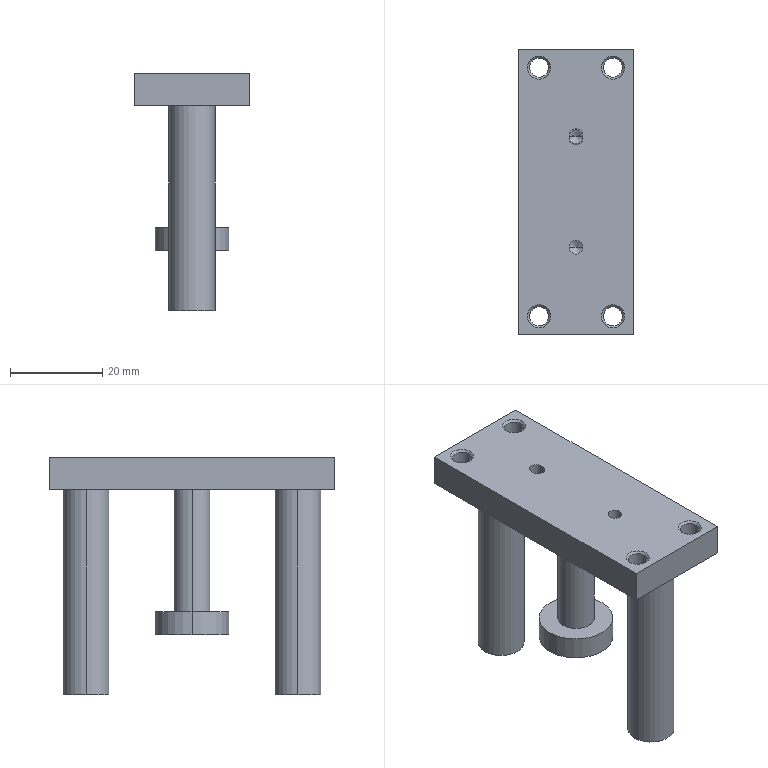Part | SolidWorks | features ICE 4, RevCut 4, RefAxis 3, HoleWzd 2, 3DProfileFeature 1, Extrusion 1, Revolution 1 | 1 solid | 56 faces | box 25 x 62 x 51.5 mm | volume 19698 mm3 | cylinder 22 | cone 20 | plane 14 | commonest cylinder face diameters 4.134 x8 3 x6 10 x4 8 x2 16 x2
STEP:
#1=CARTESIAN_POINT('',(-5.933,27.,12.567));
#2=VERTEX_POINT('',#1);
#3=CARTESIAN_POINT('',(-10.067,27.,12.567));
#4=VERTEX_POINT('',#3);
#5=CARTESIAN_POINT('',(-8.,27.,12.567));
#6=DIRECTION('',(0.,0.,-1.));
#7=DIRECTION('',(-1.,0.,0.));
#8=AXIS2_PLACEMENT_3D('',#5,#6,#7);
#9=CIRCLE('',#8,2.067);
#10=EDGE_CURVE('',#2,#4,#9,.T.);
#11=ORIENTED_EDGE('',*,*,#10,.T.);
#12=CARTESIAN_POINT('',(-10.5,27.,13.));
#13=VERTEX_POINT('',#12);
#14=CARTESIAN_POINT('',(-10.5,27.,13.));
#15=DIRECTION('',(-0.7071,0.,0.7071));
#16=VECTOR('',#15,1000.);
#17=LINE('',#14,#16);
#18=EDGE_CURVE('',#4,#13,#17,.T.);
#19=ORIENTED_EDGE('',*,*,#18,.T.);
#20=CARTESIAN_POINT('',(-5.5,27.,13.));
#21=VERTEX_POINT('',#20);
#22=CARTESIAN_POINT('',(-8.,27.,13.));
#23=DIRECTION('',(0.,0.,-1.));
#24=DIRECTION('',(-1.,0.,0.));
#25=AXIS2_PLACEMENT_3D('',#22,#23,#24);
#26=CIRCLE('',#25,2.5);
#27=EDGE_CURVE('',#21,#13,#26,.T.);
#28=ORIENTED_EDGE('',*,*,#27,.F.);
#29=CARTESIAN_POINT('',(-5.5,27.,13.));
#30=DIRECTION('',(0.7071,0.,0.7071));
#31=VECTOR('',#30,1000.);
#32=LINE('',#29,#31);
#33=EDGE_CURVE('',#2,#21,#32,.T.);
#34=ORIENTED_EDGE('',*,*,#33,.F.);
#35=EDGE_LOOP('',(#11,#19,#28,#34));
#36=FACE_OUTER_BOUND('',#35,.T.);
#37=CARTESIAN_POINT('',(-8.,27.,13.));
#38=DIRECTION('',(0.,0.,1.));
#39=DIRECTION('',(1.,0.,0.));
#40=AXIS2_PLACEMENT_3D('',#37,#38,#39);
#41=CONICAL_SURFACE('',#40,2.5,0.7854);
#42=ADVANCED_FACE('',(#36),#41,.F.);
#43=ORIENTED_EDGE('',*,*,#10,.F.);
#44=CARTESIAN_POINT('',(-5.933,27.,6.433));
#45=VERTEX_POINT('',#44);
#46=CARTESIAN_POINT('',(-5.933,27.,13.));
#47=DIRECTION('',(0.,0.,-1.));
#48=VECTOR('',#47,1000.);
#49=LINE('',#46,#48);
#50=EDGE_CURVE('',#2,#45,#49,.T.);
#51=ORIENTED_EDGE('',*,*,#50,.T.);
#52=CARTESIAN_POINT('',(-10.067,27.,6.433));
#53=VERTEX_POINT('',#52);
#54=CARTESIAN_POINT('',(-8.,27.,6.433));
#55=DIRECTION('',(0.,0.,-1.));
#56=DIRECTION('',(-1.,0.,0.));
#57=AXIS2_PLACEMENT_3D('',#54,#55,#56);
#58=CIRCLE('',#57,2.067);
#59=EDGE_CURVE('',#45,#53,#58,.T.);
#60=ORIENTED_EDGE('',*,*,#59,.T.);
#61=CARTESIAN_POINT('',(-10.067,27.,13.));
#62=DIRECTION('',(0.,0.,-1.));
#63=VECTOR('',#62,1000.);
#64=LINE('',#61,#63);
#65=EDGE_CURVE('',#4,#53,#64,.T.);
#66=ORIENTED_EDGE('',*,*,#65,.F.);
#67=EDGE_LOOP('',(#43,#51,#60,#66));
#68=FACE_OUTER_BOUND('',#67,.T.);
#69=CARTESIAN_POINT('',(-8.,27.,13.));
#70=DIRECTION('',(0.,0.,-1.));
#71=DIRECTION('',(-1.,0.,0.));
#72=AXIS2_PLACEMENT_3D('',#69,#70,#71);
#73=CYLINDRICAL_SURFACE('',#72,2.067);
#74=ADVANCED_FACE('',(#68),#73,.F.);
#75=ORIENTED_EDGE('',*,*,#59,.F.);
#76=CARTESIAN_POINT('',(-5.5,27.,6.));
#77=VERTEX_POINT('',#76);
#78=CARTESIAN_POINT('',(-5.933,27.,6.433));
#79=DIRECTION('',(0.7071,0.,-0.7071));
#80=VECTOR('',#79,1000.);
#81=LINE('',#78,#80);
#82=EDGE_CURVE('',#45,#77,#81,.T.);
#83=ORIENTED_EDGE('',*,*,#82,.T.);
#84=CARTESIAN_POINT('',(-10.5,27.,6.));
#85=VERTEX_POINT('',#84);
#86=CARTESIAN_POINT('',(-8.,27.,6.));
#87=DIRECTION('',(0.,0.,-1.));
#88=DIRECTION('',(-1.,0.,0.));
#89=AXIS2_PLACEMENT_3D('',#86,#87,#88);
#90=CIRCLE('',#89,2.5);
#91=EDGE_CURVE('',#77,#85,#90,.T.);
#92=ORIENTED_EDGE('',*,*,#91,.T.);
#93=CARTESIAN_POINT('',(-10.067,27.,6.433));
#94=DIRECTION('',(-0.7071,0.,-0.7071));
#95=VECTOR('',#94,1000.);
#96=LINE('',#93,#95);
#97=EDGE_CURVE('',#53,#85,#96,.T.);
#98=ORIENTED_EDGE('',*,*,#97,.F.);
#99=EDGE_LOOP('',(#75,#83,#92,#98));
#100=FACE_OUTER_BOUND('',#99,.T.);
#101=CARTESIAN_POINT('',(-8.,27.,6.433));
#102=DIRECTION('',(0.,0.,-1.));
#103=DIRECTION('',(-1.,0.,0.));
#104=AXIS2_PLACEMENT_3D('',#101,#102,#103);
#105=CONICAL_SURFACE('',#104,2.067,0.7854);
#106=ADVANCED_FACE('',(#100),#105,.F.);
#107=CARTESIAN_POINT('',(10.067,27.,12.567));
#108=VERTEX_POINT('',#107);
#109=CARTESIAN_POINT('',(5.933,27.,12.567));
#110=VERTEX_POINT('',#109);
#111=CARTESIAN_POINT('',(8.,27.,12.567));
#112=DIRECTION('',(0.,0.,-1.));
#113=DIRECTION('',(-1.,0.,0.));
#114=AXIS2_PLACEMENT_3D('',#111,#112,#113);
#115=CIRCLE('',#114,2.067);
#116=EDGE_CURVE('',#108,#110,#115,.T.);
#117=ORIENTED_EDGE('',*,*,#116,.T.);
#118=CARTESIAN_POINT('',(5.5,27.,13.));
#119=VERTEX_POINT('',#118);
#120=CARTESIAN_POINT('',(5.5,27.,13.));
#121=DIRECTION('',(-0.7071,0.,0.7071));
#122=VECTOR('',#121,1000.);
#123=LINE('',#120,#122);
#124=EDGE_CURVE('',#110,#119,#123,.T.);
#125=ORIENTED_EDGE('',*,*,#124,.T.);
#126=CARTESIAN_POINT('',(10.5,27.,13.));
#127=VERTEX_POINT('',#126);
#128=CARTESIAN_POINT('',(8.,27.,13.));
#129=DIRECTION('',(0.,0.,-1.));
#130=DIRECTION('',(-1.,0.,0.));
#131=AXIS2_PLACEMENT_3D('',#128,#129,#130);
#132=CIRCLE('',#131,2.5);
#133=EDGE_CURVE('',#127,#119,#132,.T.);
#134=ORIENTED_EDGE('',*,*,#133,.F.);
#135=CARTESIAN_POINT('',(10.5,27.,13.));
#136=DIRECTION('',(0.7071,0.,0.7071));
#137=VECTOR('',#136,1000.);
#138=LINE('',#135,#137);
#139=EDGE_CURVE('',#108,#127,#138,.T.);
#140=ORIENTED_EDGE('',*,*,#139,.F.);
#141=EDGE_LOOP('',(#117,#125,#134,#140));
#142=FACE_OUTER_BOUND('',#141,.T.);
#143=CARTESIAN_POINT('',(8.,27.,13.));
#144=DIRECTION('',(0.,0.,1.));
#145=DIRECTION('',(1.,0.,0.));
#146=AXIS2_PLACEMENT_3D('',#143,#144,#145);
#147=CONICAL_SURFACE('',#146,2.5,0.7854);
#148=ADVANCED_FACE('',(#142),#147,.F.);
#149=ORIENTED_EDGE('',*,*,#116,.F.);
#150=CARTESIAN_POINT('',(10.067,27.,6.433));
#151=VERTEX_POINT('',#150);
#152=CARTESIAN_POINT('',(10.067,27.,13.));
#153=DIRECTION('',(0.,0.,-1.));
#154=VECTOR('',#153,1000.);
#155=LINE('',#152,#154);
#156=EDGE_CURVE('',#108,#151,#155,.T.);
#157=ORIENTED_EDGE('',*,*,#156,.T.);
#158=CARTESIAN_POINT('',(5.933,27.,6.433));
#159=VERTEX_POINT('',#158);
#160=CARTESIAN_POINT('',(8.,27.,6.433));
#161=DIRECTION('',(0.,0.,-1.));
#162=DIRECTION('',(-1.,0.,0.));
#163=AXIS2_PLACEMENT_3D('',#160,#161,#162);
#164=CIRCLE('',#163,2.067);
#165=EDGE_CURVE('',#151,#159,#164,.T.);
#166=ORIENTED_EDGE('',*,*,#165,.T.);
#167=CARTESIAN_POINT('',(5.933,27.,13.));
#168=DIRECTION('',(0.,0.,-1.));
#169=VECTOR('',#168,1000.);
#170=LINE('',#167,#169);
#171=EDGE_CURVE('',#110,#159,#170,.T.);
#172=ORIENTED_EDGE('',*,*,#171,.F.);
#173=EDGE_LOOP('',(#149,#157,#166,#172));
#174=FACE_OUTER_BOUND('',#173,.T.);
#175=CARTESIAN_POINT('',(8.,27.,13.));
#176=DIRECTION('',(0.,0.,-1.));
#177=DIRECTION('',(-1.,0.,0.));
#178=AXIS2_PLACEMENT_3D('',#175,#176,#177);
#179=CYLINDRICAL_SURFACE('',#178,2.067);
#180=ADVANCED_FACE('',(#174),#179,.F.);
#181=ORIENTED_EDGE('',*,*,#165,.F.);
#182=CARTESIAN_POINT('',(10.5,27.,6.));
#183=VERTEX_POINT('',#182);
#184=CARTESIAN_POINT('',(10.067,27.,6.433));
#185=DIRECTION('',(0.7071,0.,-0.7071));
#186=VECTOR('',#185,1000.);
#187=LINE('',#184,#186);
#188=EDGE_CURVE('',#151,#183,#187,.T.);
#189=ORIENTED_EDGE('',*,*,#188,.T.);
#190=CARTESIAN_POINT('',(5.5,27.,6.));
#191=VERTEX_POINT('',#190);
#192=CARTESIAN_POINT('',(8.,27.,6.));
#193=DIRECTION('',(0.,0.,-1.));
#194=DIRECTION('',(-1.,0.,0.));
#195=AXIS2_PLACEMENT_3D('',#192,#193,#194);
#196=CIRCLE('',#195,2.5);
#197=EDGE_CURVE('',#183,#191,#196,.T.);
#198=ORIENTED_EDGE('',*,*,#197,.T.);
#199=CARTESIAN_POINT('',(5.933,27.,6.433));
#200=DIRECTION('',(-0.7071,0.,-0.7071));
#201=VECTOR('',#200,1000.);
#202=LINE('',#199,#201);
#203=EDGE_CURVE('',#159,#191,#202,.T.);
#204=ORIENTED_EDGE('',*,*,#203,.F.);
#205=EDGE_LOOP('',(#181,#189,#198,#204));
#206=FACE_OUTER_BOUND('',#205,.T.);
#207=CARTESIAN_POINT('',(8.,27.,6.433));
#208=DIRECTION('',(0.,0.,-1.));
#209=DIRECTION('',(-1.,0.,0.));
#210=AXIS2_PLACEMENT_3D('',#207,#208,#209);
#211=CONICAL_SURFACE('',#210,2.067,0.7854);
#212=ADVANCED_FACE('',(#206),#211,.F.);
#213=CARTESIAN_POINT('',(-5.933,-27.,12.567));
#214=VERTEX_POINT('',#213);
#215=CARTESIAN_POINT('',(-10.067,-27.,12.567));
#216=VERTEX_POINT('',#215);
#217=CARTESIAN_POINT('',(-8.,-27.,12.567));
#218=DIRECTION('',(0.,0.,-1.));
#219=DIRECTION('',(-1.,0.,0.));
#220=AXIS2_PLACEMENT_3D('',#217,#218,#219);
#221=CIRCLE('',#220,2.067);
#222=EDGE_CURVE('',#214,#216,#221,.T.);
#223=ORIENTED_EDGE('',*,*,#222,.T.);
#224=CARTESIAN_POINT('',(-10.5,-27.,13.));
#225=VERTEX_POINT('',#224);
#226=CARTESIAN_POINT('',(-10.5,-27.,13.));
#227=DIRECTION('',(-0.7071,0.,0.7071));
#228=VECTOR('',#227,1000.);
#229=LINE('',#226,#228);
#230=EDGE_CURVE('',#216,#225,#229,.T.);
#231=ORIENTED_EDGE('',*,*,#230,.T.);
#232=CARTESIAN_POINT('',(-5.5,-27.,13.));
#233=VERTEX_POINT('',#232);
#234=CARTESIAN_POINT('',(-8.,-27.,13.));
#235=DIRECTION('',(0.,0.,-1.));
#236=DIRECTION('',(-1.,0.,0.));
#237=AXIS2_PLACEMENT_3D('',#234,#235,#236);
#238=CIRCLE('',#237,2.5);
#239=EDGE_CURVE('',#233,#225,#238,.T.);
#240=ORIENTED_EDGE('',*,*,#239,.F.);
#241=CARTESIAN_POINT('',(-5.5,-27.,13.));
#242=DIRECTION('',(0.7071,0.,0.7071));
#243=VECTOR('',#242,1000.);
#244=LINE('',#241,#243);
#245=EDGE_CURVE('',#214,#233,#244,.T.);
#246=ORIENTED_EDGE('',*,*,#245,.F.);
#247=EDGE_LOOP('',(#223,#231,#240,#246));
#248=FACE_OUTER_BOUND('',#247,.T.);
#249=CARTESIAN_POINT('',(-8.,-27.,13.));
#250=DIRECTION('',(0.,0.,1.));
#251=DIRECTION('',(1.,0.,0.));
#252=AXIS2_PLACEMENT_3D('',#249,#250,#251);
#253=CONICAL_SURFACE('',#252,2.5,0.7854);
#254=ADVANCED_FACE('',(#248),#253,.F.);
#255=ORIENTED_EDGE('',*,*,#222,.F.);
#256=CARTESIAN_POINT('',(-5.933,-27.,6.433));
#257=VERTEX_POINT('',#256);
#258=CARTESIAN_POINT('',(-5.933,-27.,13.));
#259=DIRECTION('',(0.,0.,-1.));
#260=VECTOR('',#259,1000.);
#261=LINE('',#258,#260);
#262=EDGE_CURVE('',#214,#257,#261,.T.);
#263=ORIENTED_EDGE('',*,*,#262,.T.);
#264=CARTESIAN_POINT('',(-10.067,-27.,6.433));
#265=VERTEX_POINT('',#264);
#266=CARTESIAN_POINT('',(-8.,-27.,6.433));
#267=DIRECTION('',(0.,0.,-1.));
#268=DIRECTION('',(-1.,0.,0.));
#269=AXIS2_PLACEMENT_3D('',#266,#267,#268);
#270=CIRCLE('',#269,2.067);
#271=EDGE_CURVE('',#257,#265,#270,.T.);
#272=ORIENTED_EDGE('',*,*,#271,.T.);
#273=CARTESIAN_POINT('',(-10.067,-27.,13.));
#274=DIRECTION('',(0.,0.,-1.));
#275=VECTOR('',#274,1000.);
#276=LINE('',#273,#275);
#277=EDGE_CURVE('',#216,#265,#276,.T.);
#278=ORIENTED_EDGE('',*,*,#277,.F.);
#279=EDGE_LOOP('',(#255,#263,#272,#278));
#280=FACE_OUTER_BOUND('',#279,.T.);
#281=CARTESIAN_POINT('',(-8.,-27.,13.));
#282=DIRECTION('',(0.,0.,-1.));
#283=DIRECTION('',(-1.,0.,0.));
#284=AXIS2_PLACEMENT_3D('',#281,#282,#283);
#285=CYLINDRICAL_SURFACE('',#284,2.067);
#286=ADVANCED_FACE('',(#280),#285,.F.);
#287=ORIENTED_EDGE('',*,*,#271,.F.);
#288=CARTESIAN_POINT('',(-5.5,-27.,6.));
#289=VERTEX_POINT('',#288);
#290=CARTESIAN_POINT('',(-5.933,-27.,6.433));
#291=DIRECTION('',(0.7071,0.,-0.7071));
#292=VECTOR('',#291,1000.);
#293=LINE('',#290,#292);
#294=EDGE_CURVE('',#257,#289,#293,.T.);
#295=ORIENTED_EDGE('',*,*,#294,.T.);
#296=CARTESIAN_POINT('',(-10.5,-27.,6.));
#297=VERTEX_POINT('',#296);
#298=CARTESIAN_POINT('',(-8.,-27.,6.));
#299=DIRECTION('',(0.,0.,-1.));
#300=DIRECTION('',(-1.,0.,0.));
#301=AXIS2_PLACEMENT_3D('',#298,#299,#300);
#302=CIRCLE('',#301,2.5);
#303=EDGE_CURVE('',#289,#297,#302,.T.);
#304=ORIENTED_EDGE('',*,*,#303,.T.);
#305=CARTESIAN_POINT('',(-10.067,-27.,6.433));
#306=DIRECTION('',(-0.7071,0.,-0.7071));
#307=VECTOR('',#306,1000.);
#308=LINE('',#305,#307);
#309=EDGE_CURVE('',#265,#297,#308,.T.);
#310=ORIENTED_EDGE('',*,*,#309,.F.);
#311=EDGE_LOOP('',(#287,#295,#304,#310));
#312=FACE_OUTER_BOUND('',#311,.T.);
#313=CARTESIAN_POINT('',(-8.,-27.,6.433));
#314=DIRECTION('',(0.,0.,-1.));
#315=DIRECTION('',(-1.,0.,0.));
#316=AXIS2_PLACEMENT_3D('',#313,#314,#315);
#317=CONICAL_SURFACE('',#316,2.067,0.7854);
#318=ADVANCED_FACE('',(#312),#317,.F.);
#319=CARTESIAN_POINT('',(10.067,-27.,12.567));
#320=VERTEX_POINT('',#319);
#321=CARTESIAN_POINT('',(5.933,-27.,12.567));
#322=VERTEX_POINT('',#321);
#323=CARTESIAN_POINT('',(8.,-27.,12.567));
#324=DIRECTION('',(0.,0.,-1.));
#325=DIRECTION('',(-1.,0.,0.));
#326=AXIS2_PLACEMENT_3D('',#323,#324,#325);
#327=CIRCLE('',#326,2.067);
#328=EDGE_CURVE('',#320,#322,#327,.T.);
#329=ORIENTED_EDGE('',*,*,#328,.T.);
#330=CARTESIAN_POINT('',(5.5,-27.,13.));
#331=VERTEX_POINT('',#330);
#332=CARTESIAN_POINT('',(5.5,-27.,13.));
#333=DIRECTION('',(-0.7071,0.,0.7071));
#334=VECTOR('',#333,1000.);
#335=LINE('',#332,#334);
#336=EDGE_CURVE('',#322,#331,#335,.T.);
#337=ORIENTED_EDGE('',*,*,#336,.T.);
#338=CARTESIAN_POINT('',(10.5,-27.,13.));
#339=VERTEX_POINT('',#338);
#340=CARTESIAN_POINT('',(8.,-27.,13.));
#341=DIRECTION('',(0.,0.,-1.));
#342=DIRECTION('',(-1.,0.,0.));
#343=AXIS2_PLACEMENT_3D('',#340,#341,#342);
#344=CIRCLE('',#343,2.5);
#345=EDGE_CURVE('',#339,#331,#344,.T.);
#346=ORIENTED_EDGE('',*,*,#345,.F.);
#347=CARTESIAN_POINT('',(10.5,-27.,13.));
#348=DIRECTION('',(0.7071,0.,0.7071));
#349=VECTOR('',#348,1000.);
#350=LINE('',#347,#349);
#351=EDGE_CURVE('',#320,#339,#350,.T.);
#352=ORIENTED_EDGE('',*,*,#351,.F.);
#353=EDGE_LOOP('',(#329,#337,#346,#352));
#354=FACE_OUTER_BOUND('',#353,.T.);
#355=CARTESIAN_POINT('',(8.,-27.,13.));
#356=DIRECTION('',(0.,0.,1.));
#357=DIRECTION('',(1.,0.,0.));
#358=AXIS2_PLACEMENT_3D('',#355,#356,#357);
#359=CONICAL_SURFACE('',#358,2.5,0.7854);
#360=ADVANCED_FACE('',(#354),#359,.F.);
#361=ORIENTED_EDGE('',*,*,#328,.F.);
#362=CARTESIAN_POINT('',(10.067,-27.,6.433));
#363=VERTEX_POINT('',#362);
#364=CARTESIAN_POINT('',(10.067,-27.,13.));
#365=DIRECTION('',(0.,0.,-1.));
#366=VECTOR('',#365,1000.);
#367=LINE('',#364,#366);
#368=EDGE_CURVE('',#320,#363,#367,.T.);
#369=ORIENTED_EDGE('',*,*,#368,.T.);
#370=CARTESIAN_POINT('',(5.933,-27.,6.433));
#371=VERTEX_POINT('',#370);
#372=CARTESIAN_POINT('',(8.,-27.,6.433));
#373=DIRECTION('',(0.,0.,-1.));
#374=DIRECTION('',(-1.,0.,0.));
#375=AXIS2_PLACEMENT_3D('',#372,#373,#374);
#376=CIRCLE('',#375,2.067);
#377=EDGE_CURVE('',#363,#371,#376,.T.);
#378=ORIENTED_EDGE('',*,*,#377,.T.);
#379=CARTESIAN_POINT('',(5.933,-27.,13.));
#380=DIRECTION('',(0.,0.,-1.));
#381=VECTOR('',#380,1000.);
#382=LINE('',#379,#381);
#383=EDGE_CURVE('',#322,#371,#382,.T.);
#384=ORIENTED_EDGE('',*,*,#383,.F.);
#385=EDGE_LOOP('',(#361,#369,#378,#384));
#386=FACE_OUTER_BOUND('',#385,.T.);
#387=CARTESIAN_POINT('',(8.,-27.,13.));
#388=DIRECTION('',(0.,0.,-1.));
#389=DIRECTION('',(-1.,0.,0.));
#390=AXIS2_PLACEMENT_3D('',#387,#388,#389);
#391=CYLINDRICAL_SURFACE('',#390,2.067);
#392=ADVANCED_FACE('',(#386),#391,.F.);
#393=ORIENTED_EDGE('',*,*,#377,.F.);
#394=CARTESIAN_POINT('',(10.5,-27.,6.));
#395=VERTEX_POINT('',#394);
#396=CARTESIAN_POINT('',(10.067,-27.,6.433));
#397=DIRECTION('',(0.7071,0.,-0.7071));
#398=VECTOR('',#397,1000.);
#399=LINE('',#396,#398);
#400=EDGE_CURVE('',#363,#395,#399,.T.);
#401=ORIENTED_EDGE('',*,*,#400,.T.);
#402=CARTESIAN_POINT('',(5.5,-27.,6.));
#403=VERTEX_POINT('',#402);
#404=CARTESIAN_POINT('',(8.,-27.,6.));
#405=DIRECTION('',(0.,0.,-1.));
#406=DIRECTION('',(-1.,0.,0.));
#407=AXIS2_PLACEMENT_3D('',#404,#405,#406);
#408=CIRCLE('',#407,2.5);
#409=EDGE_CURVE('',#395,#403,#408,.T.);
#410=ORIENTED_EDGE('',*,*,#409,.T.);
#411=CARTESIAN_POINT('',(5.933,-27.,6.433));
#412=DIRECTION('',(-0.7071,0.,-0.7071));
#413=VECTOR('',#412,1000.);
#414=LINE('',#411,#413);
#415=EDGE_CURVE('',#371,#403,#414,.T.);
#416=ORIENTED_EDGE('',*,*,#415,.F.);
#417=EDGE_LOOP('',(#393,#401,#410,#416));
#418=FACE_OUTER_BOUND('',#417,.T.);
#419=CARTESIAN_POINT('',(8.,-27.,6.433));
#420=DIRECTION('',(0.,0.,-1.));
#421=DIRECTION('',(-1.,0.,0.));
#422=AXIS2_PLACEMENT_3D('',#419,#420,#421);
#423=CONICAL_SURFACE('',#422,2.067,0.7854);
#424=ADVANCED_FACE('',(#418),#423,.F.);
#425=CARTESIAN_POINT('',(-1.5,-12.,7.));
#426=VERTEX_POINT('',#425);
#427=CARTESIAN_POINT('',(1.5,-12.,7.));
#428=VERTEX_POINT('',#427);
#429=CARTESIAN_POINT('',(0.,-12.,7.));
#430=DIRECTION('',(0.,0.,1.));
#431=DIRECTION('',(1.,0.,0.));
#432=AXIS2_PLACEMENT_3D('',#429,#430,#431);
#433=CIRCLE('',#432,1.5);
#434=EDGE_CURVE('',#426,#428,#433,.T.);
#435=ORIENTED_EDGE('',*,*,#434,.F.);
#436=CARTESIAN_POINT('',(-1.5,-12.,13.));
#437=VERTEX_POINT('',#436);
#438=CARTESIAN_POINT('',(-1.5,-12.,13.));
#439=DIRECTION('',(0.,0.,1.));
#440=VECTOR('',#439,1000.);
#441=LINE('',#438,#440);
#442=EDGE_CURVE('',#426,#437,#441,.T.);
#443=ORIENTED_EDGE('',*,*,#442,.T.);
#444=CARTESIAN_POINT('',(1.5,-12.,13.));
#445=VERTEX_POINT('',#444);
#446=CARTESIAN_POINT('',(0.,-12.,13.));
#447=DIRECTION('',(0.,0.,1.));
#448=DIRECTION('',(1.,0.,0.));
#449=AXIS2_PLACEMENT_3D('',#446,#447,#448);
#450=CIRCLE('',#449,1.5);
#451=EDGE_CURVE('',#437,#445,#450,.T.);
#452=ORIENTED_EDGE('',*,*,#451,.T.);
#453=CARTESIAN_POINT('',(1.5,-12.,13.));
#454=DIRECTION('',(0.,0.,1.));
#455=VECTOR('',#454,1000.);
#456=LINE('',#453,#455);
#457=EDGE_CURVE('',#428,#445,#456,.T.);
#458=ORIENTED_EDGE('',*,*,#457,.F.);
#459=EDGE_LOOP('',(#435,#443,#452,#458));
#460=FACE_OUTER_BOUND('',#459,.T.);
#461=CARTESIAN_POINT('',(0.,-12.,13.));
#462=DIRECTION('',(0.,0.,1.));
#463=DIRECTION('',(1.,0.,0.));
#464=AXIS2_PLACEMENT_3D('',#461,#462,#463);
#465=CYLINDRICAL_SURFACE('',#464,1.5);
#466=ADVANCED_FACE('',(#460),#465,.F.);
#467=CARTESIAN_POINT('',(0.,-12.,6.134));
#468=VERTEX_POINT('',#467);
#469=CARTESIAN_POINT('',(1.5,-12.,7.));
#470=DIRECTION('',(0.866,0.,0.5));
#471=VECTOR('',#470,1000.);
#472=LINE('',#469,#471);
#473=EDGE_CURVE('',#468,#428,#472,.T.);
#474=ORIENTED_EDGE('',*,*,#473,.F.);
#475=CARTESIAN_POINT('',(-1.5,-12.,7.));
#476=DIRECTION('',(-0.866,0.,0.5));
#477=VECTOR('',#476,1000.);
#478=LINE('',#475,#477);
#479=EDGE_CURVE('',#468,#426,#478,.T.);
#480=ORIENTED_EDGE('',*,*,#479,.T.);
#481=ORIENTED_EDGE('',*,*,#434,.T.);
#482=EDGE_LOOP('',(#474,#480,#481));
#483=FACE_OUTER_BOUND('',#482,.T.);
#484=CARTESIAN_POINT('',(0.,-12.,7.));
#485=DIRECTION('',(0.,0.,1.));
#486=DIRECTION('',(1.,0.,0.));
#487=AXIS2_PLACEMENT_3D('',#484,#485,#486);
#488=CONICAL_SURFACE('',#487,1.5,1.047);
#489=ADVANCED_FACE('',(#483),#488,.F.);
#490=CARTESIAN_POINT('',(-1.5,12.,7.));
#491=VERTEX_POINT('',#490);
#492=CARTESIAN_POINT('',(1.5,12.,7.));
#493=VERTEX_POINT('',#492);
#494=CARTESIAN_POINT('',(0.,12.,7.));
#495=DIRECTION('',(0.,0.,1.));
#496=DIRECTION('',(1.,0.,0.));
#497=AXIS2_PLACEMENT_3D('',#494,#495,#496);
#498=CIRCLE('',#497,1.5);
#499=EDGE_CURVE('',#491,#493,#498,.T.);
#500=ORIENTED_EDGE('',*,*,#499,.F.);
#501=CARTESIAN_POINT('',(-1.5,12.,10.));
#502=VERTEX_POINT('',#501);
#503=CARTESIAN_POINT('',(-1.5,12.,13.));
#504=DIRECTION('',(0.,0.,1.));
#505=VECTOR('',#504,1000.);
#506=LINE('',#503,#505);
#507=EDGE_CURVE('',#491,#502,#506,.T.);
#508=ORIENTED_EDGE('',*,*,#507,.T.);
#509=CARTESIAN_POINT('',(1.5,12.,10.));
#510=VERTEX_POINT('',#509);
#511=CARTESIAN_POINT('',(0.,12.,10.));
#512=DIRECTION('',(0.,0.,-1.));
#513=DIRECTION('',(1.,0.,0.));
#514=AXIS2_PLACEMENT_3D('',#511,#512,#513);
#515=CIRCLE('',#514,1.5);
#516=EDGE_CURVE('',#510,#502,#515,.T.);
#517=ORIENTED_EDGE('',*,*,#516,.F.);
#518=CARTESIAN_POINT('',(1.5,12.,13.));
#519=DIRECTION('',(0.,0.,1.));
#520=VECTOR('',#519,1000.);
#521=LINE('',#518,#520);
#522=EDGE_CURVE('',#493,#510,#521,.T.);
#523=ORIENTED_EDGE('',*,*,#522,.F.);
#524=EDGE_LOOP('',(#500,#508,#517,#523));
#525=FACE_OUTER_BOUND('',#524,.T.);
#526=CARTESIAN_POINT('',(0.,12.,13.));
#527=DIRECTION('',(0.,0.,1.));
#528=DIRECTION('',(1.,0.,0.));
#529=AXIS2_PLACEMENT_3D('',#526,#527,#528);
#530=CYLINDRICAL_SURFACE('',#529,1.5);
#531=ADVANCED_FACE('',(#525),#530,.F.);
#532=CARTESIAN_POINT('',(0.,12.,6.134));
#533=VERTEX_POINT('',#532);
#534=CARTESIAN_POINT('',(1.5,12.,7.));
#535=DIRECTION('',(0.866,0.,0.5));
#536=VECTOR('',#535,1000.);
#537=LINE('',#534,#536);
#538=EDGE_CURVE('',#533,#493,#537,.T.);
#539=ORIENTED_EDGE('',*,*,#538,.F.);
#540=CARTESIAN_POINT('',(-1.5,12.,7.));
#541=DIRECTION('',(-0.866,0.,0.5));
#542=VECTOR('',#541,1000.);
#543=LINE('',#540,#542);
#544=EDGE_CURVE('',#533,#491,#543,.T.);
#545=ORIENTED_EDGE('',*,*,#544,.T.);
#546=ORIENTED_EDGE('',*,*,#499,.T.);
#547=EDGE_LOOP('',(#539,#545,#546));
#548=FACE_OUTER_BOUND('',#547,.T.);
#549=CARTESIAN_POINT('',(0.,12.,7.));
#550=DIRECTION('',(0.,0.,1.));
#551=DIRECTION('',(1.,0.,0.));
#552=AXIS2_PLACEMENT_3D('',#549,#550,#551);
#553=CONICAL_SURFACE('',#552,1.5,1.047);
#554=ADVANCED_FACE('',(#548),#553,.F.);
#555=CARTESIAN_POINT('',(8.,0.,-25.5));
#556=VERTEX_POINT('',#555);
#557=CARTESIAN_POINT('',(-8.,0.,-25.5));
#558=VERTEX_POINT('',#557);
#559=CARTESIAN_POINT('',(0.,0.,-25.5));
#560=DIRECTION('',(0.,0.,1.));
#561=DIRECTION('',(1.,0.,0.));
#562=AXIS2_PLACEMENT_3D('',#559,#560,#561);
#563=CIRCLE('',#562,8.);
#564=EDGE_CURVE('',#556,#558,#563,.T.);
#565=ORIENTED_EDGE('',*,*,#564,.T.);
#566=CARTESIAN_POINT('',(-8.,0.,-20.5));
#567=VERTEX_POINT('',#566);
#568=CARTESIAN_POINT('',(-8.,0.,-25.5));
#569=DIRECTION('',(0.,0.,1.));
#570=VECTOR('',#569,1000.);
#571=LINE('',#568,#570);
#572=EDGE_CURVE('',#558,#567,#571,.T.);
#573=ORIENTED_EDGE('',*,*,#572,.T.);
#574=CARTESIAN_POINT('',(8.,0.,-20.5));
#575=VERTEX_POINT('',#574);
#576=CARTESIAN_POINT('',(0.,0.,-20.5));
#577=DIRECTION('',(0.,0.,1.));
#578=DIRECTION('',(1.,0.,0.));
#579=AXIS2_PLACEMENT_3D('',#576,#577,#578);
#580=CIRCLE('',#579,8.);
#581=EDGE_CURVE('',#575,#567,#580,.T.);
#582=ORIENTED_EDGE('',*,*,#581,.F.);
#583=CARTESIAN_POINT('',(8.,0.,-25.5));
#584=DIRECTION('',(0.,0.,1.));
#585=VECTOR('',#584,1000.);
#586=LINE('',#583,#585);
#587=EDGE_CURVE('',#556,#575,#586,.T.);
#588=ORIENTED_EDGE('',*,*,#587,.F.);
#589=EDGE_LOOP('',(#565,#573,#582,#588));
#590=FACE_OUTER_BOUND('',#589,.T.);
#591=CARTESIAN_POINT('',(0.,0.,-25.5));
#592=DIRECTION('',(0.,0.,1.));
#593=DIRECTION('',(1.,0.,0.));
#594=AXIS2_PLACEMENT_3D('',#591,#592,#593);
#595=CYLINDRICAL_SURFACE('',#594,8.);
#596=ADVANCED_FACE('',(#590),#595,.T.);
#597=CARTESIAN_POINT('',(4.,0.,-20.5));
#598=VERTEX_POINT('',#597);
#599=CARTESIAN_POINT('',(-4.,0.,-20.5));
#600=VERTEX_POINT('',#599);
#601=CARTESIAN_POINT('',(0.,0.,-20.5));
#602=DIRECTION('',(0.,0.,1.));
#603=DIRECTION('',(1.,0.,0.));
#604=AXIS2_PLACEMENT_3D('',#601,#602,#603);
#605=CIRCLE('',#604,4.);
#606=EDGE_CURVE('',#598,#600,#605,.T.);
#607=ORIENTED_EDGE('',*,*,#606,.T.);
#608=CARTESIAN_POINT('',(-4.,0.,6.));
#609=VERTEX_POINT('',#608);
#610=CARTESIAN_POINT('',(-4.,0.,-25.5));
#611=DIRECTION('',(0.,0.,1.));
#612=VECTOR('',#611,1000.);
#613=LINE('',#610,#612);
#614=EDGE_CURVE('',#600,#609,#613,.T.);
#615=ORIENTED_EDGE('',*,*,#614,.T.);
#616=CARTESIAN_POINT('',(4.,0.,6.));
#617=VERTEX_POINT('',#616);
#618=CARTESIAN_POINT('',(0.,0.,6.));
#619=DIRECTION('',(0.,0.,-1.));
#620=DIRECTION('',(1.,0.,0.));
#621=AXIS2_PLACEMENT_3D('',#618,#619,#620);
#622=CIRCLE('',#621,4.);
#623=EDGE_CURVE('',#609,#617,#622,.T.);
#624=ORIENTED_EDGE('',*,*,#623,.T.);
#625=CARTESIAN_POINT('',(4.,0.,-25.5));
#626=DIRECTION('',(0.,0.,1.));
#627=VECTOR('',#626,1000.);
#628=LINE('',#625,#627);
#629=EDGE_CURVE('',#598,#617,#628,.T.);
#630=ORIENTED_EDGE('',*,*,#629,.F.);
#631=EDGE_LOOP('',(#607,#615,#624,#630));
#632=FACE_OUTER_BOUND('',#631,.T.);
#633=CARTESIAN_POINT('',(0.,0.,-25.5));
#634=DIRECTION('',(0.,0.,1.));
#635=DIRECTION('',(1.,0.,0.));
#636=AXIS2_PLACEMENT_3D('',#633,#634,#635);
#637=CYLINDRICAL_SURFACE('',#636,4.);
#638=ADVANCED_FACE('',(#632),#637,.T.);
#639=CARTESIAN_POINT('',(5.,-23.,-38.5));
#640=VERTEX_POINT('',#639);
#641=CARTESIAN_POINT('',(-5.,-23.,-38.5));
#642=VERTEX_POINT('',#641);
#643=CARTESIAN_POINT('',(0.,-23.,-38.5));
#644=DIRECTION('',(0.,0.,1.));
#645=DIRECTION('',(-1.,0.,0.));
#646=AXIS2_PLACEMENT_3D('',#643,#644,#645);
#647=CIRCLE('',#646,5.);
#648=EDGE_CURVE('',#640,#642,#647,.T.);
#649=ORIENTED_EDGE('',*,*,#648,.T.);
#650=CARTESIAN_POINT('',(-5.,-23.,6.));
#651=VERTEX_POINT('',#650);
#652=CARTESIAN_POINT('',(-5.,-23.,-43.));
#653=DIRECTION('',(0.,0.,1.));
#654=VECTOR('',#653,1000.);
#655=LINE('',#652,#654);
#656=EDGE_CURVE('',#642,#651,#655,.T.);
#657=ORIENTED_EDGE('',*,*,#656,.T.);
#658=CARTESIAN_POINT('',(5.,-23.,6.));
#659=VERTEX_POINT('',#658);
#660=CARTESIAN_POINT('',(0.,-23.,6.));
#661=DIRECTION('',(0.,0.,1.));
#662=DIRECTION('',(1.,0.,0.));
#663=AXIS2_PLACEMENT_3D('',#660,#661,#662);
#664=CIRCLE('',#663,5.);
#665=EDGE_CURVE('',#659,#651,#664,.T.);
#666=ORIENTED_EDGE('',*,*,#665,.F.);
#667=CARTESIAN_POINT('',(5.,-23.,-43.));
#668=DIRECTION('',(0.,0.,1.));
#669=VECTOR('',#668,1000.);
#670=LINE('',#667,#669);
#671=EDGE_CURVE('',#640,#659,#670,.T.);
#672=ORIENTED_EDGE('',*,*,#671,.F.);
#673=EDGE_LOOP('',(#649,#657,#666,#672));
#674=FACE_OUTER_BOUND('',#673,.T.);
#675=CARTESIAN_POINT('',(0.,-23.,-43.));
#676=DIRECTION('',(0.,0.,1.));
#677=DIRECTION('',(1.,0.,0.));
#678=AXIS2_PLACEMENT_3D('',#675,#676,#677);
#679=CYLINDRICAL_SURFACE('',#678,5.);
#680=ADVANCED_FACE('',(#674),#679,.T.);
#681=CARTESIAN_POINT('',(5.,23.,-38.5));
#682=VERTEX_POINT('',#681);
#683=CARTESIAN_POINT('',(-5.,23.,-38.5));
#684=VERTEX_POINT('',#683);
#685=CARTESIAN_POINT('',(0.,23.,-38.5));
#686=DIRECTION('',(0.,0.,1.));
#687=DIRECTION('',(-1.,0.,0.));
#688=AXIS2_PLACEMENT_3D('',#685,#686,#687);
#689=CIRCLE('',#688,5.);
#690=EDGE_CURVE('',#682,#684,#689,.T.);
#691=ORIENTED_EDGE('',*,*,#690,.T.);
#692=CARTESIAN_POINT('',(-5.,23.,6.));
#693=VERTEX_POINT('',#692);
#694=CARTESIAN_POINT('',(-5.,23.,-43.));
#695=DIRECTION('',(0.,0.,1.));
#696=VECTOR('',#695,1000.);
#697=LINE('',#694,#696);
#698=EDGE_CURVE('',#684,#693,#697,.T.);
#699=ORIENTED_EDGE('',*,*,#698,.T.);
#700=CARTESIAN_POINT('',(5.,23.,6.));
#701=VERTEX_POINT('',#700);
#702=CARTESIAN_POINT('',(0.,23.,6.));
#703=DIRECTION('',(0.,0.,1.));
#704=DIRECTION('',(1.,0.,0.));
#705=AXIS2_PLACEMENT_3D('',#702,#703,#704);
#706=CIRCLE('',#705,5.);
#707=EDGE_CURVE('',#701,#693,#706,.T.);
#708=ORIENTED_EDGE('',*,*,#707,.F.);
#709=CARTESIAN_POINT('',(5.,23.,-43.));
#710=DIRECTION('',(0.,0.,1.));
#711=VECTOR('',#710,1000.);
#712=LINE('',#709,#711);
#713=EDGE_CURVE('',#682,#701,#712,.T.);
#714=ORIENTED_EDGE('',*,*,#713,.F.);
#715=EDGE_LOOP('',(#691,#699,#708,#714));
#716=FACE_OUTER_BOUND('',#715,.T.);
#717=CARTESIAN_POINT('',(0.,23.,-43.));
#718=DIRECTION('',(0.,0.,1.));
#719=DIRECTION('',(1.,0.,0.));
#720=AXIS2_PLACEMENT_3D('',#717,#718,#719);
#721=CYLINDRICAL_SURFACE('',#720,5.);
#722=ADVANCED_FACE('',(#716),#721,.T.);
#723=ORIENTED_EDGE('',*,*,#698,.F.);
#724=CARTESIAN_POINT('',(0.,23.,-38.5));
#725=DIRECTION('',(0.,0.,1.));
#726=DIRECTION('',(-1.,0.,0.));
#727=AXIS2_PLACEMENT_3D('',#724,#725,#726);
#728=CIRCLE('',#727,5.);
#729=EDGE_CURVE('',#684,#682,#728,.T.);
#730=ORIENTED_EDGE('',*,*,#729,.T.);
#731=ORIENTED_EDGE('',*,*,#713,.T.);
#732=CARTESIAN_POINT('',(0.,23.,6.));
#733=DIRECTION('',(0.,0.,1.));
#734=DIRECTION('',(1.,0.,0.));
#735=AXIS2_PLACEMENT_3D('',#732,#733,#734);
#736=CIRCLE('',#735,5.);
#737=EDGE_CURVE('',#693,#701,#736,.T.);
#738=ORIENTED_EDGE('',*,*,#737,.F.);
#739=EDGE_LOOP('',(#723,#730,#731,#738));
#740=FACE_OUTER_BOUND('',#739,.T.);
#741=CARTESIAN_POINT('',(0.,23.,-43.));
#742=DIRECTION('',(0.,0.,1.));
#743=DIRECTION('',(1.,0.,0.));
#744=AXIS2_PLACEMENT_3D('',#741,#742,#743);
#745=CYLINDRICAL_SURFACE('',#744,5.);
#746=ADVANCED_FACE('',(#740),#745,.T.);
#747=ORIENTED_EDGE('',*,*,#656,.F.);
#748=CARTESIAN_POINT('',(0.,-23.,-38.5));
#749=DIRECTION('',(0.,0.,1.));
#750=DIRECTION('',(-1.,0.,0.));
#751=AXIS2_PLACEMENT_3D('',#748,#749,#750);
#752=CIRCLE('',#751,5.);
#753=EDGE_CURVE('',#642,#640,#752,.T.);
#754=ORIENTED_EDGE('',*,*,#753,.T.);
#755=ORIENTED_EDGE('',*,*,#671,.T.);
#756=CARTESIAN_POINT('',(0.,-23.,6.));
#757=DIRECTION('',(0.,0.,1.));
#758=DIRECTION('',(1.,0.,0.));
#759=AXIS2_PLACEMENT_3D('',#756,#757,#758);
#760=CIRCLE('',#759,5.);
#761=EDGE_CURVE('',#651,#659,#760,.T.);
#762=ORIENTED_EDGE('',*,*,#761,.F.);
#763=EDGE_LOOP('',(#747,#754,#755,#762));
#764=FACE_OUTER_BOUND('',#763,.T.);
#765=CARTESIAN_POINT('',(0.,-23.,-43.));
#766=DIRECTION('',(0.,0.,1.));
#767=DIRECTION('',(1.,0.,0.));
#768=AXIS2_PLACEMENT_3D('',#765,#766,#767);
#769=CYLINDRICAL_SURFACE('',#768,5.);
#770=ADVANCED_FACE('',(#764),#769,.T.);
#771=CARTESIAN_POINT('',(8.,27.,6.));
#772=DIRECTION('',(0.,0.,-1.));
#773=DIRECTION('',(-1.,0.,0.));
#774=AXIS2_PLACEMENT_3D('',#771,#772,#773);
#775=CIRCLE('',#774,2.5);
#776=EDGE_CURVE('',#191,#183,#775,.T.);
#777=ORIENTED_EDGE('',*,*,#776,.F.);
#778=ORIENTED_EDGE('',*,*,#197,.F.);
#779=EDGE_LOOP('',(#777,#778));
#780=FACE_BOUND('',#779,.T.);
#781=CARTESIAN_POINT('',(8.,-27.,6.));
#782=DIRECTION('',(0.,0.,-1.));
#783=DIRECTION('',(-1.,0.,0.));
#784=AXIS2_PLACEMENT_3D('',#781,#782,#783);
#785=CIRCLE('',#784,2.5);
#786=EDGE_CURVE('',#403,#395,#785,.T.);
#787=ORIENTED_EDGE('',*,*,#786,.F.);
#788=ORIENTED_EDGE('',*,*,#409,.F.);
#789=EDGE_LOOP('',(#787,#788));
#790=FACE_BOUND('',#789,.T.);
#791=CARTESIAN_POINT('',(12.5,31.,6.));
#792=VERTEX_POINT('',#791);
#793=CARTESIAN_POINT('',(-12.5,31.,6.));
#794=VERTEX_POINT('',#793);
#795=CARTESIAN_POINT('',(12.5,31.,6.));
#796=DIRECTION('',(-1.,0.,0.));
#797=VECTOR('',#796,1000.);
#798=LINE('',#795,#797);
#799=EDGE_CURVE('',#792,#794,#798,.T.);
#800=ORIENTED_EDGE('',*,*,#799,.F.);
#801=CARTESIAN_POINT('',(12.5,-31.,6.));
#802=VERTEX_POINT('',#801);
#803=CARTESIAN_POINT('',(12.5,-31.,6.));
#804=DIRECTION('',(0.,1.,0.));
#805=VECTOR('',#804,1000.);
#806=LINE('',#803,#805);
#807=EDGE_CURVE('',#802,#792,#806,.T.);
#808=ORIENTED_EDGE('',*,*,#807,.F.);
#809=CARTESIAN_POINT('',(-12.5,-31.,6.));
#810=VERTEX_POINT('',#809);
#811=CARTESIAN_POINT('',(-12.5,-31.,6.));
#812=DIRECTION('',(1.,0.,0.));
#813=VECTOR('',#812,1000.);
#814=LINE('',#811,#813);
#815=EDGE_CURVE('',#810,#802,#814,.T.);
#816=ORIENTED_EDGE('',*,*,#815,.F.);
#817=CARTESIAN_POINT('',(-12.5,31.,6.));
#818=DIRECTION('',(0.,-1.,0.));
#819=VECTOR('',#818,1000.);
#820=LINE('',#817,#819);
#821=EDGE_CURVE('',#794,#810,#820,.T.);
#822=ORIENTED_EDGE('',*,*,#821,.F.);
#823=EDGE_LOOP('',(#800,#808,#816,#822));
#824=FACE_OUTER_BOUND('',#823,.T.);
#825=ORIENTED_EDGE('',*,*,#707,.T.);
#826=ORIENTED_EDGE('',*,*,#737,.T.);
#827=EDGE_LOOP('',(#825,#826));
#828=FACE_BOUND('',#827,.T.);
#829=ORIENTED_EDGE('',*,*,#665,.T.);
#830=ORIENTED_EDGE('',*,*,#761,.T.);
#831=EDGE_LOOP('',(#829,#830));
#832=FACE_BOUND('',#831,.T.);
#833=CARTESIAN_POINT('',(0.,0.,6.));
#834=DIRECTION('',(0.,0.,-1.));
#835=DIRECTION('',(1.,0.,0.));
#836=AXIS2_PLACEMENT_3D('',#833,#834,#835);
#837=CIRCLE('',#836,4.);
#838=EDGE_CURVE('',#617,#609,#837,.T.);
#839=ORIENTED_EDGE('',*,*,#838,.F.);
#840=ORIENTED_EDGE('',*,*,#623,.F.);
#841=EDGE_LOOP('',(#839,#840));
#842=FACE_BOUND('',#841,.T.);
#843=CARTESIAN_POINT('',(-8.,-27.,6.));
#844=DIRECTION('',(0.,0.,-1.));
#845=DIRECTION('',(-1.,0.,0.));
#846=AXIS2_PLACEMENT_3D('',#843,#844,#845);
#847=CIRCLE('',#846,2.5);
#848=EDGE_CURVE('',#297,#289,#847,.T.);
#849=ORIENTED_EDGE('',*,*,#848,.F.);
#850=ORIENTED_EDGE('',*,*,#303,.F.);
#851=EDGE_LOOP('',(#849,#850));
#852=FACE_BOUND('',#851,.T.);
#853=CARTESIAN_POINT('',(-8.,27.,6.));
#854=DIRECTION('',(0.,0.,-1.));
#855=DIRECTION('',(-1.,0.,0.));
#856=AXIS2_PLACEMENT_3D('',#853,#854,#855);
#857=CIRCLE('',#856,2.5);
#858=EDGE_CURVE('',#85,#77,#857,.T.);
#859=ORIENTED_EDGE('',*,*,#858,.F.);
#860=ORIENTED_EDGE('',*,*,#91,.F.);
#861=EDGE_LOOP('',(#859,#860));
#862=FACE_BOUND('',#861,.T.);
#863=CARTESIAN_POINT('',(0.,0.,6.));
#864=DIRECTION('',(0.,0.,1.));
#865=DIRECTION('',(1.,0.,0.));
#866=AXIS2_PLACEMENT_3D('',#863,#864,#865);
#867=PLANE('',#866);
#868=ADVANCED_FACE('',(#780,#790,#824,#828,#832,#842,#852,#862),#867,.F.);
#869=ORIENTED_EDGE('',*,*,#133,.T.);
#870=CARTESIAN_POINT('',(8.,27.,13.));
#871=DIRECTION('',(0.,0.,-1.));
#872=DIRECTION('',(-1.,0.,0.));
#873=AXIS2_PLACEMENT_3D('',#870,#871,#872);
#874=CIRCLE('',#873,2.5);
#875=EDGE_CURVE('',#119,#127,#874,.T.);
#876=ORIENTED_EDGE('',*,*,#875,.T.);
#877=EDGE_LOOP('',(#869,#876));
#878=FACE_BOUND('',#877,.T.);
#879=ORIENTED_EDGE('',*,*,#345,.T.);
#880=CARTESIAN_POINT('',(8.,-27.,13.));
#881=DIRECTION('',(0.,0.,-1.));
#882=DIRECTION('',(-1.,0.,0.));
#883=AXIS2_PLACEMENT_3D('',#880,#881,#882);
#884=CIRCLE('',#883,2.5);
#885=EDGE_CURVE('',#331,#339,#884,.T.);
#886=ORIENTED_EDGE('',*,*,#885,.T.);
#887=EDGE_LOOP('',(#879,#886));
#888=FACE_BOUND('',#887,.T.);
#889=CARTESIAN_POINT('',(0.,-12.,13.));
#890=DIRECTION('',(0.,0.,1.));
#891=DIRECTION('',(1.,0.,0.));
#892=AXIS2_PLACEMENT_3D('',#889,#890,#891);
#893=CIRCLE('',#892,1.5);
#894=EDGE_CURVE('',#445,#437,#893,.T.);
#895=ORIENTED_EDGE('',*,*,#894,.F.);
#896=ORIENTED_EDGE('',*,*,#451,.F.);
#897=EDGE_LOOP('',(#895,#896));
#898=FACE_BOUND('',#897,.T.);
#899=CARTESIAN_POINT('',(-1.5,12.25,13.));
#900=VERTEX_POINT('',#899);
#901=CARTESIAN_POINT('',(-1.5,11.75,13.));
#902=VERTEX_POINT('',#901);
#903=CARTESIAN_POINT('',(-1.5,12.25,13.));
#904=DIRECTION('',(0.,-1.,0.));
#905=VECTOR('',#904,1000.);
#906=LINE('',#903,#905);
#907=EDGE_CURVE('',#900,#902,#906,.T.);
#908=ORIENTED_EDGE('',*,*,#907,.F.);
#909=CARTESIAN_POINT('',(1.5,12.25,13.));
#910=VERTEX_POINT('',#909);
#911=CARTESIAN_POINT('',(0.,12.25,13.));
#912=DIRECTION('',(0.,0.,1.));
#913=DIRECTION('',(1.,0.,0.));
#914=AXIS2_PLACEMENT_3D('',#911,#912,#913);
#915=CIRCLE('',#914,1.5);
#916=EDGE_CURVE('',#910,#900,#915,.T.);
#917=ORIENTED_EDGE('',*,*,#916,.F.);
#918=CARTESIAN_POINT('',(1.5,11.75,13.));
#919=VERTEX_POINT('',#918);
#920=CARTESIAN_POINT('',(1.5,11.75,13.));
#921=DIRECTION('',(0.,1.,0.));
#922=VECTOR('',#921,1000.);
#923=LINE('',#920,#922);
#924=EDGE_CURVE('',#919,#910,#923,.T.);
#925=ORIENTED_EDGE('',*,*,#924,.F.);
#926=CARTESIAN_POINT('',(0.,11.75,13.));
#927=DIRECTION('',(0.,0.,1.));
#928=DIRECTION('',(1.,0.,0.));
#929=AXIS2_PLACEMENT_3D('',#926,#927,#928);
#930=CIRCLE('',#929,1.5);
#931=EDGE_CURVE('',#902,#919,#930,.T.);
#932=ORIENTED_EDGE('',*,*,#931,.F.);
#933=EDGE_LOOP('',(#908,#917,#925,#932));
#934=FACE_BOUND('',#933,.T.);
#935=CARTESIAN_POINT('',(12.5,31.,13.));
#936=VERTEX_POINT('',#935);
#937=CARTESIAN_POINT('',(-12.5,31.,13.));
#938=VERTEX_POINT('',#937);
#939=CARTESIAN_POINT('',(12.5,31.,13.));
#940=DIRECTION('',(-1.,0.,0.));
#941=VECTOR('',#940,1000.);
#942=LINE('',#939,#941);
#943=EDGE_CURVE('',#936,#938,#942,.T.);
#944=ORIENTED_EDGE('',*,*,#943,.T.);
#945=CARTESIAN_POINT('',(-12.5,-31.,13.));
#946=VERTEX_POINT('',#945);
#947=CARTESIAN_POINT('',(-12.5,31.,13.));
#948=DIRECTION('',(0.,-1.,0.));
#949=VECTOR('',#948,1000.);
#950=LINE('',#947,#949);
#951=EDGE_CURVE('',#938,#946,#950,.T.);
#952=ORIENTED_EDGE('',*,*,#951,.T.);
#953=CARTESIAN_POINT('',(12.5,-31.,13.));
#954=VERTEX_POINT('',#953);
#955=CARTESIAN_POINT('',(-12.5,-31.,13.));
#956=DIRECTION('',(1.,0.,0.));
#957=VECTOR('',#956,1000.);
#958=LINE('',#955,#957);
#959=EDGE_CURVE('',#946,#954,#958,.T.);
#960=ORIENTED_EDGE('',*,*,#959,.T.);
#961=CARTESIAN_POINT('',(12.5,-31.,13.));
#962=DIRECTION('',(0.,1.,0.));
#963=VECTOR('',#962,1000.);
#964=LINE('',#961,#963);
#965=EDGE_CURVE('',#954,#936,#964,.T.);
#966=ORIENTED_EDGE('',*,*,#965,.T.);
#967=EDGE_LOOP('',(#944,#952,#960,#966));
#968=FACE_OUTER_BOUND('',#967,.T.);
#969=ORIENTED_EDGE('',*,*,#239,.T.);
#970=CARTESIAN_POINT('',(-8.,-27.,13.));
#971=DIRECTION('',(0.,0.,-1.));
#972=DIRECTION('',(-1.,0.,0.));
#973=AXIS2_PLACEMENT_3D('',#970,#971,#972);
#974=CIRCLE('',#973,2.5);
#975=EDGE_CURVE('',#225,#233,#974,.T.);
#976=ORIENTED_EDGE('',*,*,#975,.T.);
#977=EDGE_LOOP('',(#969,#976));
#978=FACE_BOUND('',#977,.T.);
#979=ORIENTED_EDGE('',*,*,#27,.T.);
#980=CARTESIAN_POINT('',(-8.,27.,13.));
#981=DIRECTION('',(0.,0.,-1.));
#982=DIRECTION('',(-1.,0.,0.));
#983=AXIS2_PLACEMENT_3D('',#980,#981,#982);
#984=CIRCLE('',#983,2.5);
#985=EDGE_CURVE('',#13,#21,#984,.T.);
#986=ORIENTED_EDGE('',*,*,#985,.T.);
#987=EDGE_LOOP('',(#979,#986));
#988=FACE_BOUND('',#987,.T.);
#989=CARTESIAN_POINT('',(0.,0.,13.));
#990=DIRECTION('',(0.,0.,1.));
#991=DIRECTION('',(1.,0.,0.));
#992=AXIS2_PLACEMENT_3D('',#989,#990,#991);
#993=PLANE('',#992);
#994=ADVANCED_FACE('',(#878,#888,#898,#934,#968,#978,#988),#993,.T.);
#995=ORIENTED_EDGE('',*,*,#943,.F.);
#996=CARTESIAN_POINT('',(12.5,31.,6.));
#997=DIRECTION('',(0.,0.,1.));
#998=VECTOR('',#997,1000.);
#999=LINE('',#996,#998);
#1000=EDGE_CURVE('',#792,#936,#999,.T.);
#1001=ORIENTED_EDGE('',*,*,#1000,.F.);
#1002=ORIENTED_EDGE('',*,*,#799,.T.);
#1003=CARTESIAN_POINT('',(-12.5,31.,6.));
#1004=DIRECTION('',(0.,0.,1.));
#1005=VECTOR('',#1004,1000.);
#1006=LINE('',#1003,#1005);
#1007=EDGE_CURVE('',#794,#938,#1006,.T.);
#1008=ORIENTED_EDGE('',*,*,#1007,.T.);
#1009=EDGE_LOOP('',(#995,#1001,#1002,#1008));
#1010=FACE_OUTER_BOUND('',#1009,.T.);
#1011=CARTESIAN_POINT('',(12.5,31.,6.));
#1012=DIRECTION('',(0.,1.,0.));
#1013=DIRECTION('',(0.,0.,1.));
#1014=AXIS2_PLACEMENT_3D('',#1011,#1012,#1013);
#1015=PLANE('',#1014);
#1016=ADVANCED_FACE('',(#1010),#1015,.T.);
#1017=ORIENTED_EDGE('',*,*,#965,.F.);
#1018=CARTESIAN_POINT('',(12.5,-31.,6.));
#1019=DIRECTION('',(0.,0.,1.));
#1020=VECTOR('',#1019,1000.);
#1021=LINE('',#1018,#1020);
#1022=EDGE_CURVE('',#802,#954,#1021,.T.);
#1023=ORIENTED_EDGE('',*,*,#1022,.F.);
#1024=ORIENTED_EDGE('',*,*,#807,.T.);
#1025=ORIENTED_EDGE('',*,*,#1000,.T.);
#1026=EDGE_LOOP('',(#1017,#1023,#1024,#1025));
#1027=FACE_OUTER_BOUND('',#1026,.T.);
#1028=CARTESIAN_POINT('',(12.5,-31.,6.));
#1029=DIRECTION('',(1.,0.,0.));
#1030=DIRECTION('',(0.,0.,-1.));
#1031=AXIS2_PLACEMENT_3D('',#1028,#1029,#1030);
#1032=PLANE('',#1031);
#1033=ADVANCED_FACE('',(#1027),#1032,.T.);
#1034=ORIENTED_EDGE('',*,*,#959,.F.);
#1035=CARTESIAN_POINT('',(-12.5,-31.,6.));
#1036=DIRECTION('',(0.,0.,1.));
#1037=VECTOR('',#1036,1000.);
#1038=LINE('',#1035,#1037);
#1039=EDGE_CURVE('',#810,#946,#1038,.T.);
#1040=ORIENTED_EDGE('',*,*,#1039,.F.);
#1041=ORIENTED_EDGE('',*,*,#815,.T.);
#1042=ORIENTED_EDGE('',*,*,#1022,.T.);
#1043=EDGE_LOOP('',(#1034,#1040,#1041,#1042));
#1044=FACE_OUTER_BOUND('',#1043,.T.);
#1045=CARTESIAN_POINT('',(-12.5,-31.,6.));
#1046=DIRECTION('',(0.,-1.,0.));
#1047=DIRECTION('',(0.,0.,-1.));
#1048=AXIS2_PLACEMENT_3D('',#1045,#1046,#1047);
#1049=PLANE('',#1048);
#1050=ADVANCED_FACE('',(#1044),#1049,.T.);
#1051=ORIENTED_EDGE('',*,*,#951,.F.);
#1052=ORIENTED_EDGE('',*,*,#1007,.F.);
#1053=ORIENTED_EDGE('',*,*,#821,.T.);
#1054=ORIENTED_EDGE('',*,*,#1039,.T.);
#1055=EDGE_LOOP('',(#1051,#1052,#1053,#1054));
#1056=FACE_OUTER_BOUND('',#1055,.T.);
#1057=CARTESIAN_POINT('',(-12.5,31.,6.));
#1058=DIRECTION('',(-1.,0.,0.));
#1059=DIRECTION('',(0.,0.,1.));
#1060=AXIS2_PLACEMENT_3D('',#1057,#1058,#1059);
#1061=PLANE('',#1060);
#1062=ADVANCED_FACE('',(#1056),#1061,.T.);
#1063=ORIENTED_EDGE('',*,*,#614,.F.);
#1064=CARTESIAN_POINT('',(0.,0.,-20.5));
#1065=DIRECTION('',(0.,0.,1.));
#1066=DIRECTION('',(1.,0.,0.));
#1067=AXIS2_PLACEMENT_3D('',#1064,#1065,#1066);
#1068=CIRCLE('',#1067,4.);
#1069=EDGE_CURVE('',#600,#598,#1068,.T.);
#1070=ORIENTED_EDGE('',*,*,#1069,.T.);
#1071=ORIENTED_EDGE('',*,*,#629,.T.);
#1072=ORIENTED_EDGE('',*,*,#838,.T.);
#1073=EDGE_LOOP('',(#1063,#1070,#1071,#1072));
#1074=FACE_OUTER_BOUND('',#1073,.T.);
#1075=CARTESIAN_POINT('',(0.,0.,-25.5));
#1076=DIRECTION('',(0.,0.,1.));
#1077=DIRECTION('',(1.,0.,0.));
#1078=AXIS2_PLACEMENT_3D('',#1075,#1076,#1077);
#1079=CYLINDRICAL_SURFACE('',#1078,4.);
#1080=ADVANCED_FACE('',(#1074),#1079,.T.);
#1081=ORIENTED_EDGE('',*,*,#606,.F.);
#1082=ORIENTED_EDGE('',*,*,#1069,.F.);
#1083=EDGE_LOOP('',(#1081,#1082));
#1084=FACE_BOUND('',#1083,.T.);
#1085=ORIENTED_EDGE('',*,*,#581,.T.);
#1086=CARTESIAN_POINT('',(0.,0.,-20.5));
#1087=DIRECTION('',(0.,0.,1.));
#1088=DIRECTION('',(1.,0.,0.));
#1089=AXIS2_PLACEMENT_3D('',#1086,#1087,#1088);
#1090=CIRCLE('',#1089,8.);
#1091=EDGE_CURVE('',#567,#575,#1090,.T.);
#1092=ORIENTED_EDGE('',*,*,#1091,.T.);
#1093=EDGE_LOOP('',(#1085,#1092));
#1094=FACE_OUTER_BOUND('',#1093,.T.);
#1095=CARTESIAN_POINT('',(0.,4.,-20.5));
#1096=DIRECTION('',(0.,0.,-1.));
#1097=DIRECTION('',(-1.,0.,0.));
#1098=AXIS2_PLACEMENT_3D('',#1095,#1096,#1097);
#1099=PLANE('',#1098);
#1100=ADVANCED_FACE('',(#1084,#1094),#1099,.F.);
#1101=ORIENTED_EDGE('',*,*,#572,.F.);
#1102=CARTESIAN_POINT('',(0.,0.,-25.5));
#1103=DIRECTION('',(0.,0.,1.));
#1104=DIRECTION('',(1.,0.,0.));
#1105=AXIS2_PLACEMENT_3D('',#1102,#1103,#1104);
#1106=CIRCLE('',#1105,8.);
#1107=EDGE_CURVE('',#558,#556,#1106,.T.);
#1108=ORIENTED_EDGE('',*,*,#1107,.T.);
#1109=ORIENTED_EDGE('',*,*,#587,.T.);
#1110=ORIENTED_EDGE('',*,*,#1091,.F.);
#1111=EDGE_LOOP('',(#1101,#1108,#1109,#1110));
#1112=FACE_OUTER_BOUND('',#1111,.T.);
#1113=CARTESIAN_POINT('',(0.,0.,-25.5));
#1114=DIRECTION('',(0.,0.,1.));
#1115=DIRECTION('',(1.,0.,0.));
#1116=AXIS2_PLACEMENT_3D('',#1113,#1114,#1115);
#1117=CYLINDRICAL_SURFACE('',#1116,8.);
#1118=ADVANCED_FACE('',(#1112),#1117,.T.);
#1119=ORIENTED_EDGE('',*,*,#564,.F.);
#1120=ORIENTED_EDGE('',*,*,#1107,.F.);
#1121=EDGE_LOOP('',(#1119,#1120));
#1122=FACE_OUTER_BOUND('',#1121,.T.);
#1123=CARTESIAN_POINT('',(0.,8.,-25.5));
#1124=DIRECTION('',(0.,0.,1.));
#1125=DIRECTION('',(1.,0.,0.));
#1126=AXIS2_PLACEMENT_3D('',#1123,#1124,#1125);
#1127=PLANE('',#1126);
#1128=ADVANCED_FACE('',(#1122),#1127,.F.);
#1129=ORIENTED_EDGE('',*,*,#907,.T.);
#1130=CARTESIAN_POINT('',(-1.5,11.75,10.));
#1131=VERTEX_POINT('',#1130);
#1132=CARTESIAN_POINT('',(-1.5,11.75,10.));
#1133=DIRECTION('',(0.,0.,1.));
#1134=VECTOR('',#1133,1000.);
#1135=LINE('',#1132,#1134);
#1136=EDGE_CURVE('',#1131,#902,#1135,.T.);
#1137=ORIENTED_EDGE('',*,*,#1136,.F.);
#1138=CARTESIAN_POINT('',(-1.5,12.25,10.));
#1139=DIRECTION('',(0.,-1.,0.));
#1140=VECTOR('',#1139,1000.);
#1141=LINE('',#1138,#1140);
#1142=EDGE_CURVE('',#502,#1131,#1141,.T.);
#1143=ORIENTED_EDGE('',*,*,#1142,.F.);
#1144=CARTESIAN_POINT('',(-1.5,12.25,10.));
#1145=VERTEX_POINT('',#1144);
#1146=CARTESIAN_POINT('',(-1.5,12.25,10.));
#1147=DIRECTION('',(0.,-1.,0.));
#1148=VECTOR('',#1147,1000.);
#1149=LINE('',#1146,#1148);
#1150=EDGE_CURVE('',#1145,#502,#1149,.T.);
#1151=ORIENTED_EDGE('',*,*,#1150,.F.);
#1152=CARTESIAN_POINT('',(-1.5,12.25,10.));
#1153=DIRECTION('',(0.,0.,1.));
#1154=VECTOR('',#1153,1000.);
#1155=LINE('',#1152,#1154);
#1156=EDGE_CURVE('',#1145,#900,#1155,.T.);
#1157=ORIENTED_EDGE('',*,*,#1156,.T.);
#1158=EDGE_LOOP('',(#1129,#1137,#1143,#1151,#1157));
#1159=FACE_OUTER_BOUND('',#1158,.T.);
#1160=CARTESIAN_POINT('',(-1.5,12.25,10.));
#1161=DIRECTION('',(-1.,0.,0.));
#1162=DIRECTION('',(0.,0.,1.));
#1163=AXIS2_PLACEMENT_3D('',#1160,#1161,#1162);
#1164=PLANE('',#1163);
#1165=ADVANCED_FACE('',(#1159),#1164,.F.);
#1166=ORIENTED_EDGE('',*,*,#924,.T.);
#1167=CARTESIAN_POINT('',(1.5,12.25,10.));
#1168=VERTEX_POINT('',#1167);
#1169=CARTESIAN_POINT('',(1.5,12.25,10.));
#1170=DIRECTION('',(0.,0.,1.));
#1171=VECTOR('',#1170,1000.);
#1172=LINE('',#1169,#1171);
#1173=EDGE_CURVE('',#1168,#910,#1172,.T.);
#1174=ORIENTED_EDGE('',*,*,#1173,.F.);
#1175=CARTESIAN_POINT('',(1.5,11.75,10.));
#1176=DIRECTION('',(0.,1.,0.));
#1177=VECTOR('',#1176,1000.);
#1178=LINE('',#1175,#1177);
#1179=EDGE_CURVE('',#510,#1168,#1178,.T.);
#1180=ORIENTED_EDGE('',*,*,#1179,.F.);
#1181=CARTESIAN_POINT('',(1.5,11.75,10.));
#1182=VERTEX_POINT('',#1181);
#1183=CARTESIAN_POINT('',(1.5,11.75,10.));
#1184=DIRECTION('',(0.,1.,0.));
#1185=VECTOR('',#1184,1000.);
#1186=LINE('',#1183,#1185);
#1187=EDGE_CURVE('',#1182,#510,#1186,.T.);
#1188=ORIENTED_EDGE('',*,*,#1187,.F.);
#1189=CARTESIAN_POINT('',(1.5,11.75,10.));
#1190=DIRECTION('',(0.,0.,1.));
#1191=VECTOR('',#1190,1000.);
#1192=LINE('',#1189,#1191);
#1193=EDGE_CURVE('',#1182,#919,#1192,.T.);
#1194=ORIENTED_EDGE('',*,*,#1193,.T.);
#1195=EDGE_LOOP('',(#1166,#1174,#1180,#1188,#1194));
#1196=FACE_OUTER_BOUND('',#1195,.T.);
#1197=CARTESIAN_POINT('',(1.5,11.75,10.));
#1198=DIRECTION('',(1.,0.,0.));
#1199=DIRECTION('',(0.,0.,-1.));
#1200=AXIS2_PLACEMENT_3D('',#1197,#1198,#1199);
#1201=PLANE('',#1200);
#1202=ADVANCED_FACE('',(#1196),#1201,.F.);
#1203=ORIENTED_EDGE('',*,*,#516,.T.);
#1204=ORIENTED_EDGE('',*,*,#1142,.T.);
#1205=CARTESIAN_POINT('',(0.,11.75,10.));
#1206=DIRECTION('',(0.,0.,1.));
#1207=DIRECTION('',(1.,0.,0.));
#1208=AXIS2_PLACEMENT_3D('',#1205,#1206,#1207);
#1209=CIRCLE('',#1208,1.5);
#1210=EDGE_CURVE('',#1131,#1182,#1209,.T.);
#1211=ORIENTED_EDGE('',*,*,#1210,.T.);
#1212=ORIENTED_EDGE('',*,*,#1187,.T.);
#1213=EDGE_LOOP('',(#1203,#1204,#1211,#1212));
#1214=FACE_OUTER_BOUND('',#1213,.T.);
#1215=CARTESIAN_POINT('',(0.,11.75,10.));
#1216=DIRECTION('',(0.,0.,1.));
#1217=DIRECTION('',(1.,0.,0.));
#1218=AXIS2_PLACEMENT_3D('',#1215,#1216,#1217);
#1219=PLANE('',#1218);
#1220=ADVANCED_FACE('',(#1214),#1219,.T.);
#1221=CARTESIAN_POINT('',(0.,12.,10.));
#1222=DIRECTION('',(0.,0.,-1.));
#1223=DIRECTION('',(1.,0.,0.));
#1224=AXIS2_PLACEMENT_3D('',#1221,#1222,#1223);
#1225=CIRCLE('',#1224,1.5);
#1226=EDGE_CURVE('',#502,#510,#1225,.T.);
#1227=ORIENTED_EDGE('',*,*,#1226,.T.);
#1228=ORIENTED_EDGE('',*,*,#1179,.T.);
#1229=CARTESIAN_POINT('',(0.,12.25,10.));
#1230=DIRECTION('',(0.,0.,1.));
#1231=DIRECTION('',(1.,0.,0.));
#1232=AXIS2_PLACEMENT_3D('',#1229,#1230,#1231);
#1233=CIRCLE('',#1232,1.5);
#1234=EDGE_CURVE('',#1168,#1145,#1233,.T.);
#1235=ORIENTED_EDGE('',*,*,#1234,.T.);
#1236=ORIENTED_EDGE('',*,*,#1150,.T.);
#1237=EDGE_LOOP('',(#1227,#1228,#1235,#1236));
#1238=FACE_OUTER_BOUND('',#1237,.T.);
#1239=CARTESIAN_POINT('',(0.,11.75,10.));
#1240=DIRECTION('',(0.,0.,1.));
#1241=DIRECTION('',(1.,0.,0.));
#1242=AXIS2_PLACEMENT_3D('',#1239,#1240,#1241);
#1243=PLANE('',#1242);
#1244=ADVANCED_FACE('',(#1238),#1243,.T.);
#1245=ORIENTED_EDGE('',*,*,#931,.T.);
#1246=ORIENTED_EDGE('',*,*,#1193,.F.);
#1247=ORIENTED_EDGE('',*,*,#1210,.F.);
#1248=ORIENTED_EDGE('',*,*,#1136,.T.);
#1249=EDGE_LOOP('',(#1245,#1246,#1247,#1248));
#1250=FACE_OUTER_BOUND('',#1249,.T.);
#1251=CARTESIAN_POINT('',(0.,11.75,10.));
#1252=DIRECTION('',(0.,0.,1.));
#1253=DIRECTION('',(1.,0.,0.));
#1254=AXIS2_PLACEMENT_3D('',#1251,#1252,#1253);
#1255=CYLINDRICAL_SURFACE('',#1254,1.5);
#1256=ADVANCED_FACE('',(#1250),#1255,.F.);
#1257=ORIENTED_EDGE('',*,*,#916,.T.);
#1258=ORIENTED_EDGE('',*,*,#1156,.F.);
#1259=ORIENTED_EDGE('',*,*,#1234,.F.);
#1260=ORIENTED_EDGE('',*,*,#1173,.T.);
#1261=EDGE_LOOP('',(#1257,#1258,#1259,#1260));
#1262=FACE_OUTER_BOUND('',#1261,.T.);
#1263=CARTESIAN_POINT('',(0.,12.25,10.));
#1264=DIRECTION('',(0.,0.,1.));
#1265=DIRECTION('',(1.,0.,0.));
#1266=AXIS2_PLACEMENT_3D('',#1263,#1264,#1265);
#1267=CYLINDRICAL_SURFACE('',#1266,1.5);
#1268=ADVANCED_FACE('',(#1262),#1267,.F.);
#1269=ORIENTED_EDGE('',*,*,#544,.F.);
#1270=ORIENTED_EDGE('',*,*,#538,.T.);
#1271=CARTESIAN_POINT('',(0.,12.,7.));
#1272=DIRECTION('',(0.,0.,1.));
#1273=DIRECTION('',(1.,0.,0.));
#1274=AXIS2_PLACEMENT_3D('',#1271,#1272,#1273);
#1275=CIRCLE('',#1274,1.5);
#1276=EDGE_CURVE('',#493,#491,#1275,.T.);
#1277=ORIENTED_EDGE('',*,*,#1276,.T.);
#1278=EDGE_LOOP('',(#1269,#1270,#1277));
#1279=FACE_OUTER_BOUND('',#1278,.T.);
#1280=CARTESIAN_POINT('',(0.,12.,7.));
#1281=DIRECTION('',(0.,0.,1.));
#1282=DIRECTION('',(1.,0.,0.));
#1283=AXIS2_PLACEMENT_3D('',#1280,#1281,#1282);
#1284=CONICAL_SURFACE('',#1283,1.5,1.047);
#1285=ADVANCED_FACE('',(#1279),#1284,.F.);
#1286=ORIENTED_EDGE('',*,*,#507,.F.);
#1287=ORIENTED_EDGE('',*,*,#1276,.F.);
#1288=ORIENTED_EDGE('',*,*,#522,.T.);
#1289=ORIENTED_EDGE('',*,*,#1226,.F.);
#1290=EDGE_LOOP('',(#1286,#1287,#1288,#1289));
#1291=FACE_OUTER_BOUND('',#1290,.T.);
#1292=CARTESIAN_POINT('',(0.,12.,13.));
#1293=DIRECTION('',(0.,0.,1.));
#1294=DIRECTION('',(1.,0.,0.));
#1295=AXIS2_PLACEMENT_3D('',#1292,#1293,#1294);
#1296=CYLINDRICAL_SURFACE('',#1295,1.5);
#1297=ADVANCED_FACE('',(#1291),#1296,.F.);
#1298=ORIENTED_EDGE('',*,*,#479,.F.);
#1299=ORIENTED_EDGE('',*,*,#473,.T.);
#1300=CARTESIAN_POINT('',(0.,-12.,7.));
#1301=DIRECTION('',(0.,0.,1.));
#1302=DIRECTION('',(1.,0.,0.));
#1303=AXIS2_PLACEMENT_3D('',#1300,#1301,#1302);
#1304=CIRCLE('',#1303,1.5);
#1305=EDGE_CURVE('',#428,#426,#1304,.T.);
#1306=ORIENTED_EDGE('',*,*,#1305,.T.);
#1307=EDGE_LOOP('',(#1298,#1299,#1306));
#1308=FACE_OUTER_BOUND('',#1307,.T.);
#1309=CARTESIAN_POINT('',(0.,-12.,7.));
#1310=DIRECTION('',(0.,0.,1.));
#1311=DIRECTION('',(1.,0.,0.));
#1312=AXIS2_PLACEMENT_3D('',#1309,#1310,#1311);
#1313=CONICAL_SURFACE('',#1312,1.5,1.047);
#1314=ADVANCED_FACE('',(#1308),#1313,.F.);
#1315=ORIENTED_EDGE('',*,*,#442,.F.);
#1316=ORIENTED_EDGE('',*,*,#1305,.F.);
#1317=ORIENTED_EDGE('',*,*,#457,.T.);
#1318=ORIENTED_EDGE('',*,*,#894,.T.);
#1319=EDGE_LOOP('',(#1315,#1316,#1317,#1318));
#1320=FACE_OUTER_BOUND('',#1319,.T.);
#1321=CARTESIAN_POINT('',(0.,-12.,13.));
#1322=DIRECTION('',(0.,0.,1.));
#1323=DIRECTION('',(1.,0.,0.));
#1324=AXIS2_PLACEMENT_3D('',#1321,#1322,#1323);
#1325=CYLINDRICAL_SURFACE('',#1324,1.5);
#1326=ADVANCED_FACE('',(#1320),#1325,.F.);
#1327=ORIENTED_EDGE('',*,*,#400,.F.);
#1328=CARTESIAN_POINT('',(8.,-27.,6.433));
#1329=DIRECTION('',(0.,0.,-1.));
#1330=DIRECTION('',(-1.,0.,0.));
#1331=AXIS2_PLACEMENT_3D('',#1328,#1329,#1330);
#1332=CIRCLE('',#1331,2.067);
#1333=EDGE_CURVE('',#371,#363,#1332,.T.);
#1334=ORIENTED_EDGE('',*,*,#1333,.F.);
#1335=ORIENTED_EDGE('',*,*,#415,.T.);
#1336=ORIENTED_EDGE('',*,*,#786,.T.);
#1337=EDGE_LOOP('',(#1327,#1334,#1335,#1336));
#1338=FACE_OUTER_BOUND('',#1337,.T.);
#1339=CARTESIAN_POINT('',(8.,-27.,6.433));
#1340=DIRECTION('',(0.,0.,-1.));
#1341=DIRECTION('',(-1.,0.,0.));
#1342=AXIS2_PLACEMENT_3D('',#1339,#1340,#1341);
#1343=CONICAL_SURFACE('',#1342,2.067,0.7854);
#1344=ADVANCED_FACE('',(#1338),#1343,.F.);
#1345=ORIENTED_EDGE('',*,*,#368,.F.);
#1346=CARTESIAN_POINT('',(8.,-27.,12.567));
#1347=DIRECTION('',(0.,0.,-1.));
#1348=DIRECTION('',(-1.,0.,0.));
#1349=AXIS2_PLACEMENT_3D('',#1346,#1347,#1348);
#1350=CIRCLE('',#1349,2.067);
#1351=EDGE_CURVE('',#322,#320,#1350,.T.);
#1352=ORIENTED_EDGE('',*,*,#1351,.F.);
#1353=ORIENTED_EDGE('',*,*,#383,.T.);
#1354=ORIENTED_EDGE('',*,*,#1333,.T.);
#1355=EDGE_LOOP('',(#1345,#1352,#1353,#1354));
#1356=FACE_OUTER_BOUND('',#1355,.T.);
#1357=CARTESIAN_POINT('',(8.,-27.,13.));
#1358=DIRECTION('',(0.,0.,-1.));
#1359=DIRECTION('',(-1.,0.,0.));
#1360=AXIS2_PLACEMENT_3D('',#1357,#1358,#1359);
#1361=CYLINDRICAL_SURFACE('',#1360,2.067);
#1362=ADVANCED_FACE('',(#1356),#1361,.F.);
#1363=ORIENTED_EDGE('',*,*,#336,.F.);
#1364=ORIENTED_EDGE('',*,*,#1351,.T.);
#1365=ORIENTED_EDGE('',*,*,#351,.T.);
#1366=ORIENTED_EDGE('',*,*,#885,.F.);
#1367=EDGE_LOOP('',(#1363,#1364,#1365,#1366));
#1368=FACE_OUTER_BOUND('',#1367,.T.);
#1369=CARTESIAN_POINT('',(8.,-27.,13.));
#1370=DIRECTION('',(0.,0.,1.));
#1371=DIRECTION('',(1.,0.,0.));
#1372=AXIS2_PLACEMENT_3D('',#1369,#1370,#1371);
#1373=CONICAL_SURFACE('',#1372,2.5,0.7854);
#1374=ADVANCED_FACE('',(#1368),#1373,.F.);
#1375=ORIENTED_EDGE('',*,*,#294,.F.);
#1376=CARTESIAN_POINT('',(-8.,-27.,6.433));
#1377=DIRECTION('',(0.,0.,-1.));
#1378=DIRECTION('',(-1.,0.,0.));
#1379=AXIS2_PLACEMENT_3D('',#1376,#1377,#1378);
#1380=CIRCLE('',#1379,2.067);
#1381=EDGE_CURVE('',#265,#257,#1380,.T.);
#1382=ORIENTED_EDGE('',*,*,#1381,.F.);
#1383=ORIENTED_EDGE('',*,*,#309,.T.);
#1384=ORIENTED_EDGE('',*,*,#848,.T.);
#1385=EDGE_LOOP('',(#1375,#1382,#1383,#1384));
#1386=FACE_OUTER_BOUND('',#1385,.T.);
#1387=CARTESIAN_POINT('',(-8.,-27.,6.433));
#1388=DIRECTION('',(0.,0.,-1.));
#1389=DIRECTION('',(-1.,0.,0.));
#1390=AXIS2_PLACEMENT_3D('',#1387,#1388,#1389);
#1391=CONICAL_SURFACE('',#1390,2.067,0.7854);
#1392=ADVANCED_FACE('',(#1386),#1391,.F.);
#1393=ORIENTED_EDGE('',*,*,#262,.F.);
#1394=CARTESIAN_POINT('',(-8.,-27.,12.567));
#1395=DIRECTION('',(0.,0.,-1.));
#1396=DIRECTION('',(-1.,0.,0.));
#1397=AXIS2_PLACEMENT_3D('',#1394,#1395,#1396);
#1398=CIRCLE('',#1397,2.067);
#1399=EDGE_CURVE('',#216,#214,#1398,.T.);
#1400=ORIENTED_EDGE('',*,*,#1399,.F.);
#1401=ORIENTED_EDGE('',*,*,#277,.T.);
#1402=ORIENTED_EDGE('',*,*,#1381,.T.);
#1403=EDGE_LOOP('',(#1393,#1400,#1401,#1402));
#1404=FACE_OUTER_BOUND('',#1403,.T.);
#1405=CARTESIAN_POINT('',(-8.,-27.,13.));
#1406=DIRECTION('',(0.,0.,-1.));
#1407=DIRECTION('',(-1.,0.,0.));
#1408=AXIS2_PLACEMENT_3D('',#1405,#1406,#1407);
#1409=CYLINDRICAL_SURFACE('',#1408,2.067);
#1410=ADVANCED_FACE('',(#1404),#1409,.F.);
#1411=ORIENTED_EDGE('',*,*,#230,.F.);
#1412=ORIENTED_EDGE('',*,*,#1399,.T.);
#1413=ORIENTED_EDGE('',*,*,#245,.T.);
#1414=ORIENTED_EDGE('',*,*,#975,.F.);
#1415=EDGE_LOOP('',(#1411,#1412,#1413,#1414));
#1416=FACE_OUTER_BOUND('',#1415,.T.);
#1417=CARTESIAN_POINT('',(-8.,-27.,13.));
#1418=DIRECTION('',(0.,0.,1.));
#1419=DIRECTION('',(1.,0.,0.));
#1420=AXIS2_PLACEMENT_3D('',#1417,#1418,#1419);
#1421=CONICAL_SURFACE('',#1420,2.5,0.7854);
#1422=ADVANCED_FACE('',(#1416),#1421,.F.);
#1423=ORIENTED_EDGE('',*,*,#188,.F.);
#1424=CARTESIAN_POINT('',(8.,27.,6.433));
#1425=DIRECTION('',(0.,0.,-1.));
#1426=DIRECTION('',(-1.,0.,0.));
#1427=AXIS2_PLACEMENT_3D('',#1424,#1425,#1426);
#1428=CIRCLE('',#1427,2.067);
#1429=EDGE_CURVE('',#159,#151,#1428,.T.);
#1430=ORIENTED_EDGE('',*,*,#1429,.F.);
#1431=ORIENTED_EDGE('',*,*,#203,.T.);
#1432=ORIENTED_EDGE('',*,*,#776,.T.);
#1433=EDGE_LOOP('',(#1423,#1430,#1431,#1432));
#1434=FACE_OUTER_BOUND('',#1433,.T.);
#1435=CARTESIAN_POINT('',(8.,27.,6.433));
#1436=DIRECTION('',(0.,0.,-1.));
#1437=DIRECTION('',(-1.,0.,0.));
#1438=AXIS2_PLACEMENT_3D('',#1435,#1436,#1437);
#1439=CONICAL_SURFACE('',#1438,2.067,0.7854);
#1440=ADVANCED_FACE('',(#1434),#1439,.F.);
#1441=ORIENTED_EDGE('',*,*,#156,.F.);
#1442=CARTESIAN_POINT('',(8.,27.,12.567));
#1443=DIRECTION('',(0.,0.,-1.));
#1444=DIRECTION('',(-1.,0.,0.));
#1445=AXIS2_PLACEMENT_3D('',#1442,#1443,#1444);
#1446=CIRCLE('',#1445,2.067);
#1447=EDGE_CURVE('',#110,#108,#1446,.T.);
#1448=ORIENTED_EDGE('',*,*,#1447,.F.);
#1449=ORIENTED_EDGE('',*,*,#171,.T.);
#1450=ORIENTED_EDGE('',*,*,#1429,.T.);
#1451=EDGE_LOOP('',(#1441,#1448,#1449,#1450));
#1452=FACE_OUTER_BOUND('',#1451,.T.);
#1453=CARTESIAN_POINT('',(8.,27.,13.));
#1454=DIRECTION('',(0.,0.,-1.));
#1455=DIRECTION('',(-1.,0.,0.));
#1456=AXIS2_PLACEMENT_3D('',#1453,#1454,#1455);
#1457=CYLINDRICAL_SURFACE('',#1456,2.067);
#1458=ADVANCED_FACE('',(#1452),#1457,.F.);
#1459=ORIENTED_EDGE('',*,*,#124,.F.);
#1460=ORIENTED_EDGE('',*,*,#1447,.T.);
#1461=ORIENTED_EDGE('',*,*,#139,.T.);
#1462=ORIENTED_EDGE('',*,*,#875,.F.);
#1463=EDGE_LOOP('',(#1459,#1460,#1461,#1462));
#1464=FACE_OUTER_BOUND('',#1463,.T.);
#1465=CARTESIAN_POINT('',(8.,27.,13.));
#1466=DIRECTION('',(0.,0.,1.));
#1467=DIRECTION('',(1.,0.,0.));
#1468=AXIS2_PLACEMENT_3D('',#1465,#1466,#1467);
#1469=CONICAL_SURFACE('',#1468,2.5,0.7854);
#1470=ADVANCED_FACE('',(#1464),#1469,.F.);
#1471=ORIENTED_EDGE('',*,*,#82,.F.);
#1472=CARTESIAN_POINT('',(-8.,27.,6.433));
#1473=DIRECTION('',(0.,0.,-1.));
#1474=DIRECTION('',(-1.,0.,0.));
#1475=AXIS2_PLACEMENT_3D('',#1472,#1473,#1474);
#1476=CIRCLE('',#1475,2.067);
#1477=EDGE_CURVE('',#53,#45,#1476,.T.);
#1478=ORIENTED_EDGE('',*,*,#1477,.F.);
#1479=ORIENTED_EDGE('',*,*,#97,.T.);
#1480=ORIENTED_EDGE('',*,*,#858,.T.);
#1481=EDGE_LOOP('',(#1471,#1478,#1479,#1480));
#1482=FACE_OUTER_BOUND('',#1481,.T.);
#1483=CARTESIAN_POINT('',(-8.,27.,6.433));
#1484=DIRECTION('',(0.,0.,-1.));
#1485=DIRECTION('',(-1.,0.,0.));
#1486=AXIS2_PLACEMENT_3D('',#1483,#1484,#1485);
#1487=CONICAL_SURFACE('',#1486,2.067,0.7854);
#1488=ADVANCED_FACE('',(#1482),#1487,.F.);
#1489=ORIENTED_EDGE('',*,*,#50,.F.);
#1490=CARTESIAN_POINT('',(-8.,27.,12.567));
#1491=DIRECTION('',(0.,0.,-1.));
#1492=DIRECTION('',(-1.,0.,0.));
#1493=AXIS2_PLACEMENT_3D('',#1490,#1491,#1492);
#1494=CIRCLE('',#1493,2.067);
#1495=EDGE_CURVE('',#4,#2,#1494,.T.);
#1496=ORIENTED_EDGE('',*,*,#1495,.F.);
#1497=ORIENTED_EDGE('',*,*,#65,.T.);
#1498=ORIENTED_EDGE('',*,*,#1477,.T.);
#1499=EDGE_LOOP('',(#1489,#1496,#1497,#1498));
#1500=FACE_OUTER_BOUND('',#1499,.T.);
#1501=CARTESIAN_POINT('',(-8.,27.,13.));
#1502=DIRECTION('',(0.,0.,-1.));
#1503=DIRECTION('',(-1.,0.,0.));
#1504=AXIS2_PLACEMENT_3D('',#1501,#1502,#1503);
#1505=CYLINDRICAL_SURFACE('',#1504,2.067);
#1506=ADVANCED_FACE('',(#1500),#1505,.F.);
#1507=ORIENTED_EDGE('',*,*,#18,.F.);
#1508=ORIENTED_EDGE('',*,*,#1495,.T.);
#1509=ORIENTED_EDGE('',*,*,#33,.T.);
#1510=ORIENTED_EDGE('',*,*,#985,.F.);
#1511=EDGE_LOOP('',(#1507,#1508,#1509,#1510));
#1512=FACE_OUTER_BOUND('',#1511,.T.);
#1513=CARTESIAN_POINT('',(-8.,27.,13.));
#1514=DIRECTION('',(0.,0.,1.));
#1515=DIRECTION('',(1.,0.,0.));
#1516=AXIS2_PLACEMENT_3D('',#1513,#1514,#1515);
#1517=CONICAL_SURFACE('',#1516,2.5,0.7854);
#1518=ADVANCED_FACE('',(#1512),#1517,.F.);
#1519=ORIENTED_EDGE('',*,*,#648,.F.);
#1520=ORIENTED_EDGE('',*,*,#753,.F.);
#1521=EDGE_LOOP('',(#1519,#1520));
#1522=FACE_OUTER_BOUND('',#1521,.T.);
#1523=CARTESIAN_POINT('',(0.,0.,-38.5));
#1524=DIRECTION('',(0.,0.,-1.));
#1525=DIRECTION('',(-1.,0.,0.));
#1526=AXIS2_PLACEMENT_3D('',#1523,#1524,#1525);
#1527=PLANE('',#1526);
#1528=ADVANCED_FACE('',(#1522),#1527,.T.);
#1529=ORIENTED_EDGE('',*,*,#690,.F.);
#1530=ORIENTED_EDGE('',*,*,#729,.F.);
#1531=EDGE_LOOP('',(#1529,#1530));
#1532=FACE_OUTER_BOUND('',#1531,.T.);
#1533=CARTESIAN_POINT('',(0.,0.,-38.5));
#1534=DIRECTION('',(0.,0.,-1.));
#1535=DIRECTION('',(-1.,0.,0.));
#1536=AXIS2_PLACEMENT_3D('',#1533,#1534,#1535);
#1537=PLANE('',#1536);
#1538=ADVANCED_FACE('',(#1532),#1537,.T.);
#1539=CLOSED_SHELL('',(#42,#74,#106,#148,#180,#212,#254,#286,#318,#360,#392,#424,#466,#489,#531,#554,#596,#638,#680,#722,#746,#770,#868,#994,#1016,#1033,#1050,#1062,#1080,#1100,#1118,#1128,#1165,#1202,#1220,#1244,#1256,#1268,#1285,#1297,#1314,#1326,#1344,#1362,#1374,#1392,#1410,#1422,#1440,#1458,#1470,#1488,#1506,#1518,#1528,#1538));
#1540=MANIFOLD_SOLID_BREP('',#1539);
#1541=CARTESIAN_POINT('',(0.,0.,0.));
#1542=DIRECTION('',(0.,0.,1.));
#1543=DIRECTION('',(1.,0.,0.));
#1544=AXIS2_PLACEMENT_3D('',#1541,#1542,#1543);
#1545=(LENGTH_UNIT()NAMED_UNIT(*)SI_UNIT(.MILLI.,.METRE.));
#1546=UNCERTAINTY_MEASURE_WITH_UNIT(LENGTH_MEASURE(0.00001),#1545,'','');
#1547=(NAMED_UNIT(*)PLANE_ANGLE_UNIT()SI_UNIT($,.RADIAN.));
#1548=(NAMED_UNIT(*)SI_UNIT($,.STERADIAN.)SOLID_ANGLE_UNIT());
#1549=(GEOMETRIC_REPRESENTATION_CONTEXT(3)GLOBAL_UNCERTAINTY_ASSIGNED_CONTEXT((#1546))GLOBAL_UNIT_ASSIGNED_CONTEXT((#1545,#1547,#1548))REPRESENTATION_CONTEXT('',''));
#1550=ADVANCED_BREP_SHAPE_REPRESENTATION('',(#1540,#1544),#1549);